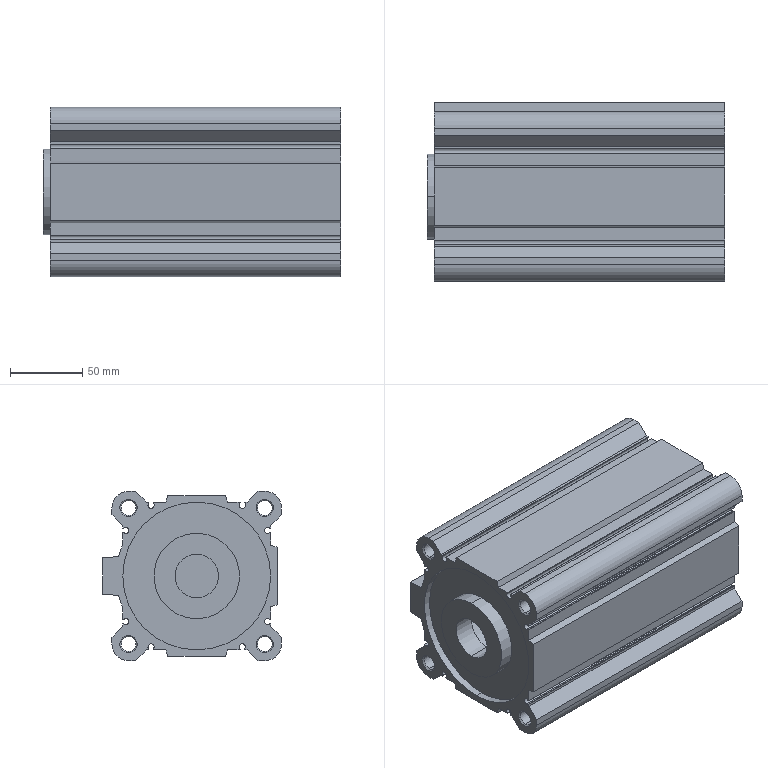Part | STEP file | 1 solid | 159 faces | box 205.5 x 123.5 x 117 mm | volume 1275384 mm3 | plane 77 | cylinder 62 | cone 20 | commonest cylinder face diameters 4.26 x18 10.106 x16 12 x8 14.95 x4 23 x4 102 x4